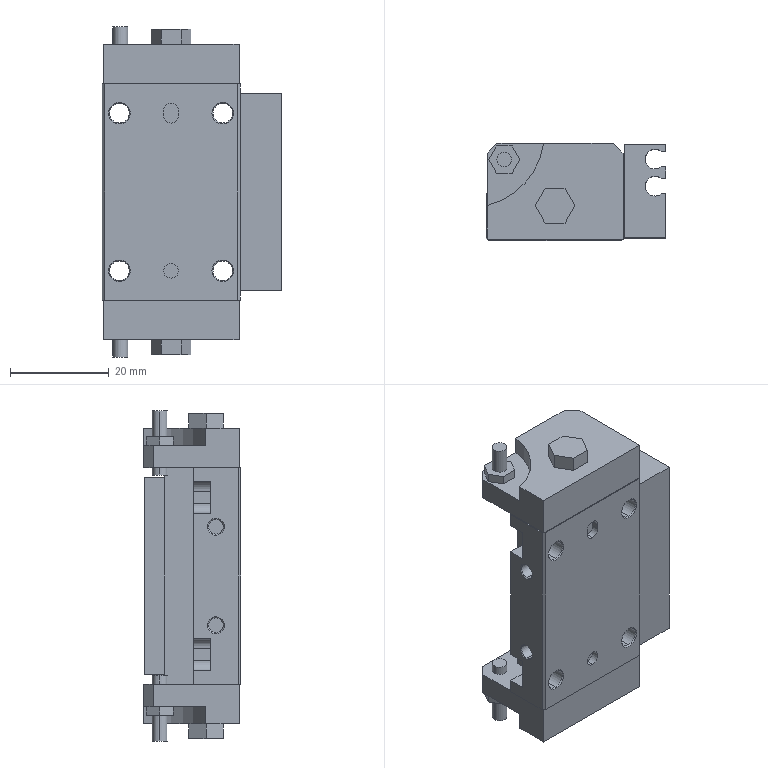Part | NX | 1 solid | 186 faces | box 36.5 x 19.7 x 67 mm | volume 26909 mm3 | plane 111 | cylinder 47 | cone 28 | commonest cylinder face diameters 3 x21 4 x20 5 x4 30 x2